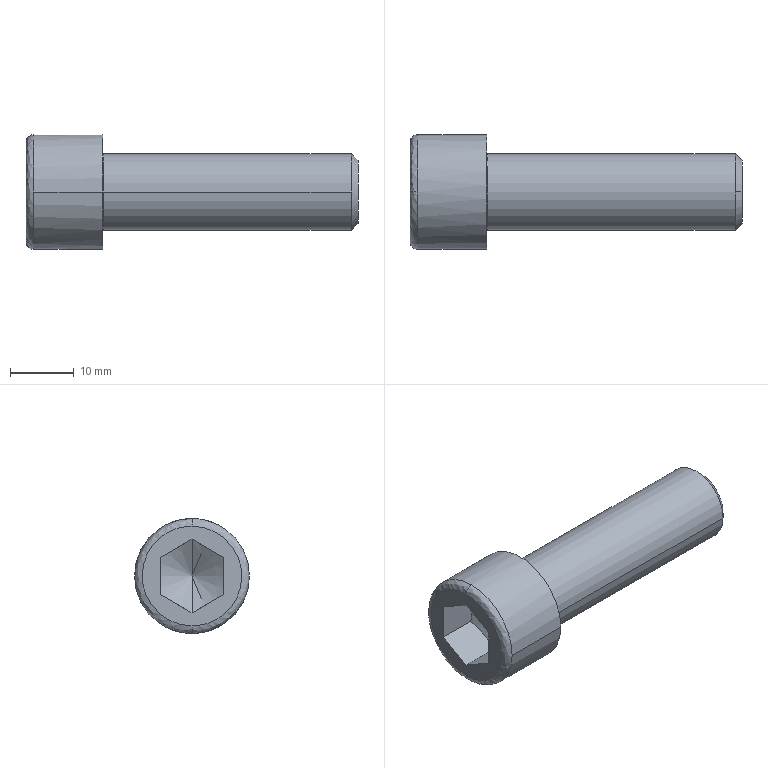Part | SolidWorks | features BaseBody 1 | 1 solid | 21 faces | box 52 x 18 x 18 mm | volume 6907 mm3 | plane 9 | spline 4 | cylinder 4 | cone 4 | commonest cylinder face diameters 12 x2 18 x2
STEP:
#1=CARTESIAN_POINT('',(0.,0.,6.1));
#2=VERTEX_POINT('',#1);
#3=CARTESIAN_POINT('',(0.,0.,-6.1));
#4=VERTEX_POINT('',#3);
#5=CARTESIAN_POINT('',(0.,0.,6.1));
#6=CARTESIAN_POINT('',(0.,0.1864,6.1));
#7=CARTESIAN_POINT('',(0.,0.4649,6.087));
#8=CARTESIAN_POINT('',(0.,0.788,6.05));
#9=CARTESIAN_POINT('',(0.,0.9492,6.026));
#10=CARTESIAN_POINT('',(0.,1.018,6.014));
#11=CARTESIAN_POINT('',(0.,1.064,6.007));
#12=CARTESIAN_POINT('',(0.,1.086,6.003));
#13=CARTESIAN_POINT('',(0.,1.304,5.962));
#14=CARTESIAN_POINT('',(0.,1.592,5.894));
#15=CARTESIAN_POINT('',(0.,1.921,5.791));
#16=CARTESIAN_POINT('',(0.,2.06,5.742));
#17=CARTESIAN_POINT('',(0.,2.153,5.708));
#18=CARTESIAN_POINT('',(0.,2.198,5.691));
#19=CARTESIAN_POINT('',(0.,2.437,5.596));
#20=CARTESIAN_POINT('',(0.,2.717,5.468));
#21=CARTESIAN_POINT('',(0.,2.987,5.32));
#22=CARTESIAN_POINT('',(0.,3.164,5.216));
#23=CARTESIAN_POINT('',(0.,3.25,5.163));
#24=CARTESIAN_POINT('',(0.,3.69,4.875));
#25=CARTESIAN_POINT('',(0.,4.016,4.611));
#26=CARTESIAN_POINT('',(0.,4.462,4.165));
#27=CARTESIAN_POINT('',(0.,4.673,3.931));
#28=CARTESIAN_POINT('',(0.,4.897,3.641));
#29=CARTESIAN_POINT('',(0.,4.988,3.512));
#30=CARTESIAN_POINT('',(0.,5.047,3.426));
#31=CARTESIAN_POINT('',(0.,5.077,3.381));
#32=CARTESIAN_POINT('',(0.,5.218,3.166));
#33=CARTESIAN_POINT('',(0.,5.374,2.9));
#34=CARTESIAN_POINT('',(0.,5.531,2.577));
#35=CARTESIAN_POINT('',(0.,5.593,2.436));
#36=CARTESIAN_POINT('',(0.,5.633,2.341));
#37=CARTESIAN_POINT('',(0.,5.654,2.291));
#38=CARTESIAN_POINT('',(0.,5.744,2.062));
#39=CARTESIAN_POINT('',(0.,5.84,1.782));
#40=CARTESIAN_POINT('',(0.,5.927,1.448));
#41=CARTESIAN_POINT('',(0.,5.965,1.28));
#42=CARTESIAN_POINT('',(0.,5.979,1.207));
#43=CARTESIAN_POINT('',(0.,5.989,1.159));
#44=CARTESIAN_POINT('',(0.,5.994,1.133));
#45=CARTESIAN_POINT('',(0.,6.066,0.7429));
#46=CARTESIAN_POINT('',(0.,6.1,0.3729));
#47=CARTESIAN_POINT('',(0.,6.1,-0.1865));
#48=CARTESIAN_POINT('',(0.,6.091,-0.3725));
#49=CARTESIAN_POINT('',(0.,6.066,-0.65));
#50=CARTESIAN_POINT('',(0.,6.05,-0.7884));
#51=CARTESIAN_POINT('',(0.,6.026,-0.9494));
#52=CARTESIAN_POINT('',(0.,6.014,-1.018));
#53=CARTESIAN_POINT('',(0.,6.007,-1.064));
#54=CARTESIAN_POINT('',(0.,6.003,-1.086));
#55=CARTESIAN_POINT('',(0.,5.962,-1.304));
#56=CARTESIAN_POINT('',(0.,5.894,-1.592));
#57=CARTESIAN_POINT('',(0.,5.791,-1.921));
#58=CARTESIAN_POINT('',(0.,5.742,-2.06));
#59=CARTESIAN_POINT('',(0.,5.708,-2.153));
#60=CARTESIAN_POINT('',(0.,5.691,-2.198));
#61=CARTESIAN_POINT('',(0.,5.596,-2.437));
#62=CARTESIAN_POINT('',(0.,5.468,-2.717));
#63=CARTESIAN_POINT('',(0.,5.32,-2.987));
#64=CARTESIAN_POINT('',(0.,5.216,-3.164));
#65=CARTESIAN_POINT('',(0.,5.163,-3.25));
#66=CARTESIAN_POINT('',(0.,4.875,-3.69));
#67=CARTESIAN_POINT('',(0.,4.611,-4.016));
#68=CARTESIAN_POINT('',(0.,4.165,-4.462));
#69=CARTESIAN_POINT('',(0.,3.931,-4.673));
#70=CARTESIAN_POINT('',(0.,3.641,-4.897));
#71=CARTESIAN_POINT('',(0.,3.512,-4.988));
#72=CARTESIAN_POINT('',(0.,3.426,-5.047));
#73=CARTESIAN_POINT('',(0.,3.381,-5.077));
#74=CARTESIAN_POINT('',(0.,3.166,-5.218));
#75=CARTESIAN_POINT('',(0.,2.9,-5.374));
#76=CARTESIAN_POINT('',(0.,2.577,-5.531));
#77=CARTESIAN_POINT('',(0.,2.436,-5.593));
#78=CARTESIAN_POINT('',(0.,2.341,-5.633));
#79=CARTESIAN_POINT('',(0.,2.291,-5.654));
#80=CARTESIAN_POINT('',(0.,2.062,-5.744));
#81=CARTESIAN_POINT('',(0.,1.782,-5.84));
#82=CARTESIAN_POINT('',(0.,1.448,-5.927));
#83=CARTESIAN_POINT('',(0.,1.28,-5.965));
#84=CARTESIAN_POINT('',(0.,1.207,-5.979));
#85=CARTESIAN_POINT('',(0.,1.159,-5.989));
#86=CARTESIAN_POINT('',(0.,1.133,-5.994));
#87=CARTESIAN_POINT('',(0.,0.7435,-6.066));
#88=CARTESIAN_POINT('',(0.,0.3728,-6.1));
#89=CARTESIAN_POINT('',(0.,0.,-6.1));
#90=B_SPLINE_CURVE_WITH_KNOTS('',3,(#5,#6,#7,#8,#9,#10,#11,#12,#13,#14,#15,#16,#17,#18,#19,#20,#21,#22,#23,#24,#25,#26,#27,#28,#29,#30,#31,#32,#33,#34,#35,#36,#37,#38,#39,#40,#41,#42,#43,#44,#45,#46,#47,#48,#49,#50,#51,#52,#53,#54,#55,#56,#57,#58,#59,#60,#61,#62,#63,#64,#65,#66,#67,#68,#69,#70,#71,#72,#73,#74,#75,#76,#77,#78,#79,#80,#81,#82,#83,#84,#85,#86,#87,#88,#89),.UNSPECIFIED.,.F.,.F.,(4,1,1,1,2,2,1,1,2,2,1,2,2,2,1,1,2,2,1,1,2,2,1,1,1,2,2,2,2,1,1,2,2,1,1,2,2,1,2,2,2,1,1,2,2,1,1,2,2,1,1,1,2,2,4),(0.75,0.7656,0.7734,0.7773,0.7793,0.7812,0.7969,0.8047,0.8086,0.8125,0.8281,0.8359,0.8437,0.875,0.8906,0.8984,0.9023,0.9063,0.9219,0.9297,0.9336,0.9375,0.9531,0.9609,0.9648,0.9668,0.9688,1.,1.016,1.023,1.027,1.029,1.031,1.047,1.055,1.059,1.063,1.078,1.086,1.094,1.125,1.141,1.148,1.152,1.156,1.172,1.18,1.184,1.188,1.203,1.211,1.215,1.217,1.219,1.25),.UNSPECIFIED.);
#91=EDGE_CURVE('',#2,#4,#90,.T.);
#92=ORIENTED_EDGE('',*,*,#91,.F.);
#93=CARTESIAN_POINT('',(0.1,0.,6.));
#94=VERTEX_POINT('',#93);
#95=CARTESIAN_POINT('',(0.1,0.,6.1));
#96=DIRECTION('',(0.,-1.,0.));
#97=DIRECTION('',(0.,0.,1.));
#98=AXIS2_PLACEMENT_3D('',#95,#96,#97);
#99=CIRCLE('',#98,0.1);
#100=EDGE_CURVE('',#2,#94,#99,.T.);
#101=ORIENTED_EDGE('',*,*,#100,.T.);
#102=CARTESIAN_POINT('',(0.1,6.,0.));
#103=VERTEX_POINT('',#102);
#104=CARTESIAN_POINT('',(0.1,0.,0.));
#105=DIRECTION('',(1.,0.,0.));
#106=DIRECTION('',(0.,1.,0.));
#107=AXIS2_PLACEMENT_3D('',#104,#105,#106);
#108=CIRCLE('',#107,6.);
#109=EDGE_CURVE('',#103,#94,#108,.T.);
#110=ORIENTED_EDGE('',*,*,#109,.F.);
#111=CARTESIAN_POINT('',(0.1,0.,-6.));
#112=VERTEX_POINT('',#111);
#113=CARTESIAN_POINT('',(0.1,0.,0.));
#114=DIRECTION('',(1.,0.,0.));
#115=DIRECTION('',(0.,1.,0.));
#116=AXIS2_PLACEMENT_3D('',#113,#114,#115);
#117=CIRCLE('',#116,6.);
#118=EDGE_CURVE('',#112,#103,#117,.T.);
#119=ORIENTED_EDGE('',*,*,#118,.F.);
#120=CARTESIAN_POINT('',(0.1,0.,-6.1));
#121=DIRECTION('',(0.,1.,0.));
#122=DIRECTION('',(0.,0.,-1.));
#123=AXIS2_PLACEMENT_3D('',#120,#121,#122);
#124=CIRCLE('',#123,0.1);
#125=EDGE_CURVE('',#4,#112,#124,.T.);
#126=ORIENTED_EDGE('',*,*,#125,.F.);
#127=EDGE_LOOP('',(#92,#101,#110,#119,#126));
#128=FACE_OUTER_BOUND('',#127,.T.);
#129=CARTESIAN_POINT('',(0.,0.,-6.1));
#130=CARTESIAN_POINT('',(0.,12.2,-6.1));
#131=CARTESIAN_POINT('',(0.,12.2,6.1));
#132=CARTESIAN_POINT('',(0.,0.,6.1));
#133=CARTESIAN_POINT('',(0.,0.,-6.041));
#134=CARTESIAN_POINT('',(0.,12.083,-6.041));
#135=CARTESIAN_POINT('',(0.,12.083,6.041));
#136=CARTESIAN_POINT('',(0.,0.,6.041));
#137=CARTESIAN_POINT('',(0.04142,0.,-6.));
#138=CARTESIAN_POINT('',(0.04142,12.,-6.));
#139=CARTESIAN_POINT('',(0.04142,12.,6.));
#140=CARTESIAN_POINT('',(0.04142,0.,6.));
#141=CARTESIAN_POINT('',(0.1,0.,-6.));
#142=CARTESIAN_POINT('',(0.1,12.,-6.));
#143=CARTESIAN_POINT('',(0.1,12.,6.));
#144=CARTESIAN_POINT('',(0.1,0.,6.));
#145=(BOUNDED_SURFACE()B_SPLINE_SURFACE(3,3,((#129,#130,#131,#132),(#133,#134,#135,#136),(#137,#138,#139,#140),(#141,#142,#143,#144)),.UNSPECIFIED.,.F.,.F.,.F.)B_SPLINE_SURFACE_WITH_KNOTS((4,4),(4,4),(0.,1.),(0.,1.),.UNSPECIFIED.)GEOMETRIC_REPRESENTATION_ITEM()RATIONAL_B_SPLINE_SURFACE(((1.,0.3333,0.3333,1.),(0.8047,0.2682,0.2682,0.8047),(0.8047,0.2682,0.2682,0.8047),(1.,0.3333,0.3333,1.)))REPRESENTATION_ITEM('')SURFACE());
#146=ADVANCED_FACE('',(#128),#145,.F.);
#147=CARTESIAN_POINT('',(-10.8,0.,9.));
#148=VERTEX_POINT('',#147);
#149=CARTESIAN_POINT('',(-10.8,-9.,0.));
#150=VERTEX_POINT('',#149);
#151=CARTESIAN_POINT('',(-10.8,0.,0.));
#152=DIRECTION('',(1.,0.,0.));
#153=DIRECTION('',(0.,1.,0.));
#154=AXIS2_PLACEMENT_3D('',#151,#152,#153);
#155=CIRCLE('',#154,9.);
#156=EDGE_CURVE('',#148,#150,#155,.T.);
#157=ORIENTED_EDGE('',*,*,#156,.F.);
#158=CARTESIAN_POINT('',(-12.,0.,7.8));
#159=VERTEX_POINT('',#158);
#160=CARTESIAN_POINT('',(-10.8,0.,7.8));
#161=DIRECTION('',(0.,-1.,0.));
#162=DIRECTION('',(0.,0.,1.));
#163=AXIS2_PLACEMENT_3D('',#160,#161,#162);
#164=CIRCLE('',#163,1.2);
#165=EDGE_CURVE('',#148,#159,#164,.T.);
#166=ORIENTED_EDGE('',*,*,#165,.T.);
#167=CARTESIAN_POINT('',(-12.,0.,-7.8));
#168=VERTEX_POINT('',#167);
#169=CARTESIAN_POINT('',(-12.,0.,7.8));
#170=CARTESIAN_POINT('',(-12.,-15.6,7.8));
#171=CARTESIAN_POINT('',(-12.,-15.6,-7.8));
#172=CARTESIAN_POINT('',(-12.,0.,-7.8));
#173=(BOUNDED_CURVE()B_SPLINE_CURVE(3,(#169,#170,#171,#172),.UNSPECIFIED.,.F.,.F.)B_SPLINE_CURVE_WITH_KNOTS((4,4),(0.25,0.75),.UNSPECIFIED.)CURVE()GEOMETRIC_REPRESENTATION_ITEM()RATIONAL_B_SPLINE_CURVE((1.,0.3333,0.3333,1.))REPRESENTATION_ITEM(''));
#174=EDGE_CURVE('',#159,#168,#173,.T.);
#175=ORIENTED_EDGE('',*,*,#174,.T.);
#176=CARTESIAN_POINT('',(-10.8,0.,-9.));
#177=VERTEX_POINT('',#176);
#178=CARTESIAN_POINT('',(-10.8,0.,-7.8));
#179=DIRECTION('',(0.,1.,0.));
#180=DIRECTION('',(0.,0.,-1.));
#181=AXIS2_PLACEMENT_3D('',#178,#179,#180);
#182=CIRCLE('',#181,1.2);
#183=EDGE_CURVE('',#177,#168,#182,.T.);
#184=ORIENTED_EDGE('',*,*,#183,.F.);
#185=CARTESIAN_POINT('',(-10.8,0.,0.));
#186=DIRECTION('',(1.,0.,0.));
#187=DIRECTION('',(0.,1.,0.));
#188=AXIS2_PLACEMENT_3D('',#185,#186,#187);
#189=CIRCLE('',#188,9.);
#190=EDGE_CURVE('',#150,#177,#189,.T.);
#191=ORIENTED_EDGE('',*,*,#190,.F.);
#192=EDGE_LOOP('',(#157,#166,#175,#184,#191));
#193=FACE_OUTER_BOUND('',#192,.T.);
#194=CARTESIAN_POINT('',(-10.8,0.,9.));
#195=CARTESIAN_POINT('',(-10.8,-18.,9.));
#196=CARTESIAN_POINT('',(-10.8,-18.,-9.));
#197=CARTESIAN_POINT('',(-10.8,0.,-9.));
#198=CARTESIAN_POINT('',(-11.503,0.,9.));
#199=CARTESIAN_POINT('',(-11.503,-18.,9.));
#200=CARTESIAN_POINT('',(-11.503,-18.,-9.));
#201=CARTESIAN_POINT('',(-11.503,0.,-9.));
#202=CARTESIAN_POINT('',(-12.,0.,8.503));
#203=CARTESIAN_POINT('',(-12.,-17.006,8.503));
#204=CARTESIAN_POINT('',(-12.,-17.006,-8.503));
#205=CARTESIAN_POINT('',(-12.,0.,-8.503));
#206=CARTESIAN_POINT('',(-12.,0.,7.8));
#207=CARTESIAN_POINT('',(-12.,-15.6,7.8));
#208=CARTESIAN_POINT('',(-12.,-15.6,-7.8));
#209=CARTESIAN_POINT('',(-12.,0.,-7.8));
#210=(BOUNDED_SURFACE()B_SPLINE_SURFACE(3,3,((#194,#195,#196,#197),(#198,#199,#200,#201),(#202,#203,#204,#205),(#206,#207,#208,#209)),.UNSPECIFIED.,.F.,.F.,.F.)B_SPLINE_SURFACE_WITH_KNOTS((4,4),(4,4),(0.,1.),(0.,1.),.UNSPECIFIED.)GEOMETRIC_REPRESENTATION_ITEM()RATIONAL_B_SPLINE_SURFACE(((1.,0.3333,0.3333,1.),(0.8047,0.2682,0.2682,0.8047),(0.8047,0.2682,0.2682,0.8047),(1.,0.3333,0.3333,1.)))REPRESENTATION_ITEM('')SURFACE());
#211=ADVANCED_FACE('',(#193),#210,.T.);
#212=ORIENTED_EDGE('',*,*,#109,.T.);
#213=CARTESIAN_POINT('',(0.1,-6.,0.));
#214=VERTEX_POINT('',#213);
#215=CARTESIAN_POINT('',(0.1,0.,0.));
#216=DIRECTION('',(1.,0.,0.));
#217=DIRECTION('',(0.,1.,0.));
#218=AXIS2_PLACEMENT_3D('',#215,#216,#217);
#219=CIRCLE('',#218,6.);
#220=EDGE_CURVE('',#94,#214,#219,.T.);
#221=ORIENTED_EDGE('',*,*,#220,.T.);
#222=CARTESIAN_POINT('',(38.926,-6.,0.));
#223=VERTEX_POINT('',#222);
#224=CARTESIAN_POINT('',(25.,-6.,0.));
#225=DIRECTION('',(1.,0.,0.));
#226=VECTOR('',#225,1000.);
#227=LINE('',#224,#226);
#228=EDGE_CURVE('',#214,#223,#227,.T.);
#229=ORIENTED_EDGE('',*,*,#228,.T.);
#230=CARTESIAN_POINT('',(38.926,0.,6.));
#231=VERTEX_POINT('',#230);
#232=CARTESIAN_POINT('',(38.926,0.,0.));
#233=DIRECTION('',(-1.,0.,0.));
#234=DIRECTION('',(0.,1.,0.));
#235=AXIS2_PLACEMENT_3D('',#232,#233,#234);
#236=CIRCLE('',#235,6.);
#237=EDGE_CURVE('',#223,#231,#236,.T.);
#238=ORIENTED_EDGE('',*,*,#237,.T.);
#239=CARTESIAN_POINT('',(38.926,6.,0.));
#240=VERTEX_POINT('',#239);
#241=CARTESIAN_POINT('',(38.926,0.,0.));
#242=DIRECTION('',(-1.,0.,0.));
#243=DIRECTION('',(0.,1.,0.));
#244=AXIS2_PLACEMENT_3D('',#241,#242,#243);
#245=CIRCLE('',#244,6.);
#246=EDGE_CURVE('',#231,#240,#245,.T.);
#247=ORIENTED_EDGE('',*,*,#246,.T.);
#248=CARTESIAN_POINT('',(25.,6.,0.));
#249=DIRECTION('',(1.,0.,0.));
#250=VECTOR('',#249,1000.);
#251=LINE('',#248,#250);
#252=EDGE_CURVE('',#103,#240,#251,.T.);
#253=ORIENTED_EDGE('',*,*,#252,.F.);
#254=EDGE_LOOP('',(#212,#221,#229,#238,#247,#253));
#255=FACE_OUTER_BOUND('',#254,.T.);
#256=CARTESIAN_POINT('',(25.,0.,0.));
#257=DIRECTION('',(1.,0.,0.));
#258=DIRECTION('',(0.,1.,0.));
#259=AXIS2_PLACEMENT_3D('',#256,#257,#258);
#260=CYLINDRICAL_SURFACE('',#259,6.);
#261=ADVANCED_FACE('',(#255),#260,.T.);
#262=CARTESIAN_POINT('',(40.,0.,4.926));
#263=VERTEX_POINT('',#262);
#264=CARTESIAN_POINT('',(40.,0.,-4.926));
#265=VERTEX_POINT('',#264);
#266=CARTESIAN_POINT('',(40.,0.,0.));
#267=DIRECTION('',(-1.,0.,0.));
#268=DIRECTION('',(0.,0.,1.));
#269=AXIS2_PLACEMENT_3D('',#266,#267,#268);
#270=CIRCLE('',#269,4.926);
#271=EDGE_CURVE('',#263,#265,#270,.T.);
#272=ORIENTED_EDGE('',*,*,#271,.T.);
#273=CARTESIAN_POINT('',(38.926,0.,-6.));
#274=VERTEX_POINT('',#273);
#275=CARTESIAN_POINT('',(38.926,0.,-6.));
#276=DIRECTION('',(-0.7071,0.,-0.7071));
#277=VECTOR('',#276,1000.);
#278=LINE('',#275,#277);
#279=EDGE_CURVE('',#265,#274,#278,.T.);
#280=ORIENTED_EDGE('',*,*,#279,.T.);
#281=CARTESIAN_POINT('',(38.926,0.,0.));
#282=DIRECTION('',(-1.,0.,0.));
#283=DIRECTION('',(0.,1.,0.));
#284=AXIS2_PLACEMENT_3D('',#281,#282,#283);
#285=CIRCLE('',#284,6.);
#286=EDGE_CURVE('',#240,#274,#285,.T.);
#287=ORIENTED_EDGE('',*,*,#286,.F.);
#288=ORIENTED_EDGE('',*,*,#246,.F.);
#289=CARTESIAN_POINT('',(38.926,0.,6.));
#290=DIRECTION('',(-0.7071,0.,0.7071));
#291=VECTOR('',#290,1000.);
#292=LINE('',#289,#291);
#293=EDGE_CURVE('',#263,#231,#292,.T.);
#294=ORIENTED_EDGE('',*,*,#293,.F.);
#295=EDGE_LOOP('',(#272,#280,#287,#288,#294));
#296=FACE_OUTER_BOUND('',#295,.T.);
#297=CARTESIAN_POINT('',(38.926,0.,0.));
#298=DIRECTION('',(-1.,0.,0.));
#299=DIRECTION('',(0.,0.,1.));
#300=AXIS2_PLACEMENT_3D('',#297,#298,#299);
#301=CONICAL_SURFACE('',#300,6.,0.7854);
#302=ADVANCED_FACE('',(#296),#301,.T.);
#303=CARTESIAN_POINT('',(-10.8,9.,0.));
#304=VERTEX_POINT('',#303);
#305=CARTESIAN_POINT('',(-10.8,0.,0.));
#306=DIRECTION('',(1.,0.,0.));
#307=DIRECTION('',(0.,1.,0.));
#308=AXIS2_PLACEMENT_3D('',#305,#306,#307);
#309=CIRCLE('',#308,9.);
#310=EDGE_CURVE('',#304,#148,#309,.T.);
#311=ORIENTED_EDGE('',*,*,#310,.T.);
#312=ORIENTED_EDGE('',*,*,#156,.T.);
#313=CARTESIAN_POINT('',(0.,-9.,0.));
#314=VERTEX_POINT('',#313);
#315=CARTESIAN_POINT('',(-6.,-9.,0.));
#316=DIRECTION('',(1.,0.,0.));
#317=VECTOR('',#316,1000.);
#318=LINE('',#315,#317);
#319=EDGE_CURVE('',#150,#314,#318,.T.);
#320=ORIENTED_EDGE('',*,*,#319,.T.);
#321=CARTESIAN_POINT('',(0.,9.,0.));
#322=VERTEX_POINT('',#321);
#323=CARTESIAN_POINT('',(0.,0.,0.));
#324=DIRECTION('',(1.,0.,0.));
#325=DIRECTION('',(0.,1.,0.));
#326=AXIS2_PLACEMENT_3D('',#323,#324,#325);
#327=CIRCLE('',#326,9.);
#328=EDGE_CURVE('',#322,#314,#327,.T.);
#329=ORIENTED_EDGE('',*,*,#328,.F.);
#330=CARTESIAN_POINT('',(-6.,9.,0.));
#331=DIRECTION('',(1.,0.,0.));
#332=VECTOR('',#331,1000.);
#333=LINE('',#330,#332);
#334=EDGE_CURVE('',#304,#322,#333,.T.);
#335=ORIENTED_EDGE('',*,*,#334,.F.);
#336=EDGE_LOOP('',(#311,#312,#320,#329,#335));
#337=FACE_OUTER_BOUND('',#336,.T.);
#338=CARTESIAN_POINT('',(-6.,0.,0.));
#339=DIRECTION('',(1.,0.,0.));
#340=DIRECTION('',(0.,1.,0.));
#341=AXIS2_PLACEMENT_3D('',#338,#339,#340);
#342=CYLINDRICAL_SURFACE('',#341,9.);
#343=ADVANCED_FACE('',(#337),#342,.T.);
#344=CARTESIAN_POINT('',(-2.667,0.,0.));
#345=VERTEX_POINT('',#344);
#346=CARTESIAN_POINT('',(-6.,0.,5.774));
#347=VERTEX_POINT('',#346);
#348=CARTESIAN_POINT('',(-6.02,0.,5.808));
#349=DIRECTION('',(-0.5,0.,0.866));
#350=VECTOR('',#349,1000.);
#351=LINE('',#348,#350);
#352=EDGE_CURVE('',#345,#347,#351,.T.);
#353=ORIENTED_EDGE('',*,*,#352,.F.);
#354=CARTESIAN_POINT('',(-6.,0.,-5.774));
#355=VERTEX_POINT('',#354);
#356=CARTESIAN_POINT('',(-6.02,0.,-5.808));
#357=DIRECTION('',(-0.5,0.,-0.866));
#358=VECTOR('',#357,1000.);
#359=LINE('',#356,#358);
#360=EDGE_CURVE('',#345,#355,#359,.T.);
#361=ORIENTED_EDGE('',*,*,#360,.T.);
#362=CARTESIAN_POINT('',(-6.,-5.,-2.887));
#363=VERTEX_POINT('',#362);
#364=CARTESIAN_POINT('',(-6.,0.,-5.774));
#365=CARTESIAN_POINT('',(-5.728,-0.8164,-5.302));
#366=CARTESIAN_POINT('',(-5.554,-1.645,-4.824));
#367=CARTESIAN_POINT('',(-5.553,-2.708,-4.21));
#368=CARTESIAN_POINT('',(-5.564,-2.921,-4.087));
#369=CARTESIAN_POINT('',(-5.604,-3.344,-3.843));
#370=CARTESIAN_POINT('',(-5.635,-3.554,-3.722));
#371=CARTESIAN_POINT('',(-5.751,-4.179,-3.361));
#372=CARTESIAN_POINT('',(-5.864,-4.591,-3.123));
#373=CARTESIAN_POINT('',(-6.,-5.,-2.887));
#374=B_SPLINE_CURVE_WITH_KNOTS('',3,(#364,#365,#366,#367,#368,#369,#370,#371,#372,#373),.UNSPECIFIED.,.F.,.F.,(4,2,2,2,4),(0.,0.002915,0.003644,0.004373,0.005831),.UNSPECIFIED.);
#375=EDGE_CURVE('',#355,#363,#374,.T.);
#376=ORIENTED_EDGE('',*,*,#375,.T.);
#377=CARTESIAN_POINT('',(-6.,-5.,2.887));
#378=VERTEX_POINT('',#377);
#379=CARTESIAN_POINT('',(-6.,-5.,-2.887));
#380=CARTESIAN_POINT('',(-5.728,-5.,-1.944));
#381=CARTESIAN_POINT('',(-5.554,-5.,-0.9872));
#382=CARTESIAN_POINT('',(-5.553,-5.,0.2399));
#383=CARTESIAN_POINT('',(-5.564,-5.,0.4865));
#384=CARTESIAN_POINT('',(-5.604,-5.,0.9743));
#385=CARTESIAN_POINT('',(-5.635,-5.,1.216));
#386=CARTESIAN_POINT('',(-5.751,-5.,1.939));
#387=CARTESIAN_POINT('',(-5.864,-5.,2.415));
#388=CARTESIAN_POINT('',(-6.,-5.,2.887));
#389=B_SPLINE_CURVE_WITH_KNOTS('',3,(#379,#380,#381,#382,#383,#384,#385,#386,#387,#388),.UNSPECIFIED.,.F.,.F.,(4,2,2,2,4),(0.,0.002915,0.003644,0.004373,0.005831),.UNSPECIFIED.);
#390=EDGE_CURVE('',#363,#378,#389,.T.);
#391=ORIENTED_EDGE('',*,*,#390,.T.);
#392=CARTESIAN_POINT('',(-6.,-5.,2.887));
#393=CARTESIAN_POINT('',(-5.728,-4.184,3.358));
#394=CARTESIAN_POINT('',(-5.554,-3.355,3.837));
#395=CARTESIAN_POINT('',(-5.553,-2.292,4.45));
#396=CARTESIAN_POINT('',(-5.564,-2.079,4.573));
#397=CARTESIAN_POINT('',(-5.604,-1.656,4.817));
#398=CARTESIAN_POINT('',(-5.635,-1.446,4.938));
#399=CARTESIAN_POINT('',(-5.751,-0.8208,5.3));
#400=CARTESIAN_POINT('',(-5.864,-0.4087,5.538));
#401=CARTESIAN_POINT('',(-6.,0.,5.774));
#402=B_SPLINE_CURVE_WITH_KNOTS('',3,(#392,#393,#394,#395,#396,#397,#398,#399,#400,#401),.UNSPECIFIED.,.F.,.F.,(4,2,2,2,4),(0.,0.002915,0.003644,0.004373,0.005831),.UNSPECIFIED.);
#403=EDGE_CURVE('',#378,#347,#402,.T.);
#404=ORIENTED_EDGE('',*,*,#403,.T.);
#405=EDGE_LOOP('',(#353,#361,#376,#391,#404));
#406=FACE_OUTER_BOUND('',#405,.T.);
#407=CARTESIAN_POINT('',(-6.02,0.,0.));
#408=DIRECTION('',(-1.,0.,0.));
#409=DIRECTION('',(0.,0.,1.));
#410=AXIS2_PLACEMENT_3D('',#407,#408,#409);
#411=CONICAL_SURFACE('',#410,5.808,1.047);
#412=ADVANCED_FACE('',(#406),#411,.F.);
#413=ORIENTED_EDGE('',*,*,#228,.F.);
#414=CARTESIAN_POINT('',(0.1,0.,0.));
#415=DIRECTION('',(1.,0.,0.));
#416=DIRECTION('',(0.,1.,0.));
#417=AXIS2_PLACEMENT_3D('',#414,#415,#416);
#418=CIRCLE('',#417,6.);
#419=EDGE_CURVE('',#214,#112,#418,.T.);
#420=ORIENTED_EDGE('',*,*,#419,.T.);
#421=ORIENTED_EDGE('',*,*,#118,.T.);
#422=ORIENTED_EDGE('',*,*,#252,.T.);
#423=ORIENTED_EDGE('',*,*,#286,.T.);
#424=CARTESIAN_POINT('',(38.926,0.,0.));
#425=DIRECTION('',(-1.,0.,0.));
#426=DIRECTION('',(0.,1.,0.));
#427=AXIS2_PLACEMENT_3D('',#424,#425,#426);
#428=CIRCLE('',#427,6.);
#429=EDGE_CURVE('',#274,#223,#428,.T.);
#430=ORIENTED_EDGE('',*,*,#429,.T.);
#431=EDGE_LOOP('',(#413,#420,#421,#422,#423,#430));
#432=FACE_OUTER_BOUND('',#431,.T.);
#433=CARTESIAN_POINT('',(25.,0.,0.));
#434=DIRECTION('',(1.,0.,0.));
#435=DIRECTION('',(0.,1.,0.));
#436=AXIS2_PLACEMENT_3D('',#433,#434,#435);
#437=CYLINDRICAL_SURFACE('',#436,6.);
#438=ADVANCED_FACE('',(#432),#437,.T.);
#439=ORIENTED_EDGE('',*,*,#100,.F.);
#440=CARTESIAN_POINT('',(0.,0.,-6.1));
#441=CARTESIAN_POINT('',(0.,-0.1864,-6.1));
#442=CARTESIAN_POINT('',(0.,-0.4649,-6.087));
#443=CARTESIAN_POINT('',(0.,-0.788,-6.05));
#444=CARTESIAN_POINT('',(0.,-0.9492,-6.026));
#445=CARTESIAN_POINT('',(0.,-1.018,-6.014));
#446=CARTESIAN_POINT('',(0.,-1.064,-6.007));
#447=CARTESIAN_POINT('',(0.,-1.086,-6.003));
#448=CARTESIAN_POINT('',(0.,-1.304,-5.962));
#449=CARTESIAN_POINT('',(0.,-1.592,-5.894));
#450=CARTESIAN_POINT('',(0.,-1.921,-5.791));
#451=CARTESIAN_POINT('',(0.,-2.06,-5.742));
#452=CARTESIAN_POINT('',(0.,-2.153,-5.708));
#453=CARTESIAN_POINT('',(0.,-2.198,-5.691));
#454=CARTESIAN_POINT('',(0.,-2.437,-5.596));
#455=CARTESIAN_POINT('',(0.,-2.717,-5.468));
#456=CARTESIAN_POINT('',(0.,-2.987,-5.32));
#457=CARTESIAN_POINT('',(0.,-3.164,-5.216));
#458=CARTESIAN_POINT('',(0.,-3.25,-5.163));
#459=CARTESIAN_POINT('',(0.,-3.69,-4.875));
#460=CARTESIAN_POINT('',(0.,-4.016,-4.611));
#461=CARTESIAN_POINT('',(0.,-4.462,-4.165));
#462=CARTESIAN_POINT('',(0.,-4.673,-3.931));
#463=CARTESIAN_POINT('',(0.,-4.897,-3.641));
#464=CARTESIAN_POINT('',(0.,-4.988,-3.512));
#465=CARTESIAN_POINT('',(0.,-5.047,-3.426));
#466=CARTESIAN_POINT('',(0.,-5.077,-3.381));
#467=CARTESIAN_POINT('',(0.,-5.218,-3.166));
#468=CARTESIAN_POINT('',(0.,-5.374,-2.9));
#469=CARTESIAN_POINT('',(0.,-5.531,-2.577));
#470=CARTESIAN_POINT('',(0.,-5.593,-2.436));
#471=CARTESIAN_POINT('',(0.,-5.633,-2.341));
#472=CARTESIAN_POINT('',(0.,-5.654,-2.291));
#473=CARTESIAN_POINT('',(0.,-5.744,-2.062));
#474=CARTESIAN_POINT('',(0.,-5.84,-1.782));
#475=CARTESIAN_POINT('',(0.,-5.927,-1.448));
#476=CARTESIAN_POINT('',(0.,-5.965,-1.28));
#477=CARTESIAN_POINT('',(0.,-5.979,-1.207));
#478=CARTESIAN_POINT('',(0.,-5.989,-1.159));
#479=CARTESIAN_POINT('',(0.,-5.994,-1.133));
#480=CARTESIAN_POINT('',(0.,-6.066,-0.7435));
#481=CARTESIAN_POINT('',(0.,-6.1,-0.3728));
#482=CARTESIAN_POINT('',(0.,-6.1,0.1864));
#483=CARTESIAN_POINT('',(0.,-6.087,0.4649));
#484=CARTESIAN_POINT('',(0.,-6.05,0.788));
#485=CARTESIAN_POINT('',(0.,-6.026,0.9492));
#486=CARTESIAN_POINT('',(0.,-6.014,1.018));
#487=CARTESIAN_POINT('',(0.,-6.007,1.064));
#488=CARTESIAN_POINT('',(0.,-6.003,1.086));
#489=CARTESIAN_POINT('',(0.,-5.962,1.304));
#490=CARTESIAN_POINT('',(0.,-5.894,1.592));
#491=CARTESIAN_POINT('',(0.,-5.791,1.921));
#492=CARTESIAN_POINT('',(0.,-5.742,2.06));
#493=CARTESIAN_POINT('',(0.,-5.708,2.153));
#494=CARTESIAN_POINT('',(0.,-5.691,2.198));
#495=CARTESIAN_POINT('',(0.,-5.596,2.437));
#496=CARTESIAN_POINT('',(0.,-5.468,2.717));
#497=CARTESIAN_POINT('',(0.,-5.32,2.987));
#498=CARTESIAN_POINT('',(0.,-5.216,3.164));
#499=CARTESIAN_POINT('',(0.,-5.163,3.25));
#500=CARTESIAN_POINT('',(0.,-4.875,3.69));
#501=CARTESIAN_POINT('',(0.,-4.611,4.016));
#502=CARTESIAN_POINT('',(0.,-4.165,4.462));
#503=CARTESIAN_POINT('',(0.,-3.931,4.673));
#504=CARTESIAN_POINT('',(0.,-3.641,4.897));
#505=CARTESIAN_POINT('',(0.,-3.512,4.988));
#506=CARTESIAN_POINT('',(0.,-3.426,5.047));
#507=CARTESIAN_POINT('',(0.,-3.381,5.077));
#508=CARTESIAN_POINT('',(0.,-3.166,5.218));
#509=CARTESIAN_POINT('',(0.,-2.9,5.374));
#510=CARTESIAN_POINT('',(0.,-2.577,5.531));
#511=CARTESIAN_POINT('',(0.,-2.436,5.593));
#512=CARTESIAN_POINT('',(0.,-2.341,5.633));
#513=CARTESIAN_POINT('',(0.,-2.291,5.654));
#514=CARTESIAN_POINT('',(0.,-2.062,5.744));
#515=CARTESIAN_POINT('',(0.,-1.782,5.84));
#516=CARTESIAN_POINT('',(0.,-1.448,5.927));
#517=CARTESIAN_POINT('',(0.,-1.28,5.965));
#518=CARTESIAN_POINT('',(0.,-1.207,5.979));
#519=CARTESIAN_POINT('',(0.,-1.159,5.989));
#520=CARTESIAN_POINT('',(0.,-1.133,5.994));
#521=CARTESIAN_POINT('',(0.,-0.7435,6.066));
#522=CARTESIAN_POINT('',(0.,-0.3728,6.1));
#523=CARTESIAN_POINT('',(0.,0.,6.1));
#524=B_SPLINE_CURVE_WITH_KNOTS('',3,(#440,#441,#442,#443,#444,#445,#446,#447,#448,#449,#450,#451,#452,#453,#454,#455,#456,#457,#458,#459,#460,#461,#462,#463,#464,#465,#466,#467,#468,#469,#470,#471,#472,#473,#474,#475,#476,#477,#478,#479,#480,#481,#482,#483,#484,#485,#486,#487,#488,#489,#490,#491,#492,#493,#494,#495,#496,#497,#498,#499,#500,#501,#502,#503,#504,#505,#506,#507,#508,#509,#510,#511,#512,#513,#514,#515,#516,#517,#518,#519,#520,#521,#522,#523),.UNSPECIFIED.,.F.,.F.,(4,1,1,1,2,2,1,1,2,2,1,2,2,2,1,1,2,2,1,1,2,2,1,1,1,2,2,2,1,1,1,2,2,1,1,2,2,1,2,2,2,1,1,2,2,1,1,2,2,1,1,1,2,2,4),(0.25,0.2656,0.2734,0.2773,0.2793,0.2813,0.2969,0.3047,0.3086,0.3125,0.3281,0.3359,0.3437,0.375,0.3906,0.3984,0.4023,0.4062,0.4219,0.4297,0.4336,0.4375,0.4531,0.4609,0.4648,0.4668,0.4687,0.5,0.5156,0.5234,0.5273,0.5293,0.5312,0.5469,0.5547,0.5586,0.5625,0.5781,0.5859,0.5937,0.625,0.6406,0.6484,0.6523,0.6562,0.6719,0.6797,0.6836,0.6875,0.7031,0.7109,0.7148,0.7168,0.7187,0.75),.UNSPECIFIED.);
#525=EDGE_CURVE('',#4,#2,#524,.T.);
#526=ORIENTED_EDGE('',*,*,#525,.F.);
#527=ORIENTED_EDGE('',*,*,#125,.T.);
#528=ORIENTED_EDGE('',*,*,#419,.F.);
#529=ORIENTED_EDGE('',*,*,#220,.F.);
#530=EDGE_LOOP('',(#439,#526,#527,#528,#529));
#531=FACE_OUTER_BOUND('',#530,.T.);
#532=CARTESIAN_POINT('',(0.,0.,6.1));
#533=CARTESIAN_POINT('',(0.,-12.2,6.1));
#534=CARTESIAN_POINT('',(0.,-12.2,-6.1));
#535=CARTESIAN_POINT('',(0.,0.,-6.1));
#536=CARTESIAN_POINT('',(0.,0.,6.041));
#537=CARTESIAN_POINT('',(0.,-12.083,6.041));
#538=CARTESIAN_POINT('',(0.,-12.083,-6.041));
#539=CARTESIAN_POINT('',(0.,0.,-6.041));
#540=CARTESIAN_POINT('',(0.04142,0.,6.));
#541=CARTESIAN_POINT('',(0.04142,-12.,6.));
#542=CARTESIAN_POINT('',(0.04142,-12.,-6.));
#543=CARTESIAN_POINT('',(0.04142,0.,-6.));
#544=CARTESIAN_POINT('',(0.1,0.,6.));
#545=CARTESIAN_POINT('',(0.1,-12.,6.));
#546=CARTESIAN_POINT('',(0.1,-12.,-6.));
#547=CARTESIAN_POINT('',(0.1,0.,-6.));
#548=(BOUNDED_SURFACE()B_SPLINE_SURFACE(3,3,((#532,#533,#534,#535),(#536,#537,#538,#539),(#540,#541,#542,#543),(#544,#545,#546,#547)),.UNSPECIFIED.,.F.,.F.,.T.)B_SPLINE_SURFACE_WITH_KNOTS((4,4),(4,4),(0.,1.),(0.,1.),.UNSPECIFIED.)GEOMETRIC_REPRESENTATION_ITEM()RATIONAL_B_SPLINE_SURFACE(((1.,0.3333,0.3333,1.),(0.8047,0.2682,0.2682,0.8047),(0.8047,0.2682,0.2682,0.8047),(1.,0.3333,0.3333,1.)))REPRESENTATION_ITEM('')SURFACE());
#549=ADVANCED_FACE('',(#531),#548,.F.);
#550=ORIENTED_EDGE('',*,*,#279,.F.);
#551=CARTESIAN_POINT('',(40.,0.,0.));
#552=DIRECTION('',(-1.,0.,0.));
#553=DIRECTION('',(0.,0.,1.));
#554=AXIS2_PLACEMENT_3D('',#551,#552,#553);
#555=CIRCLE('',#554,4.926);
#556=EDGE_CURVE('',#265,#263,#555,.T.);
#557=ORIENTED_EDGE('',*,*,#556,.T.);
#558=ORIENTED_EDGE('',*,*,#293,.T.);
#559=ORIENTED_EDGE('',*,*,#237,.F.);
#560=ORIENTED_EDGE('',*,*,#429,.F.);
#561=EDGE_LOOP('',(#550,#557,#558,#559,#560));
#562=FACE_OUTER_BOUND('',#561,.T.);
#563=CARTESIAN_POINT('',(38.926,0.,0.));
#564=DIRECTION('',(-1.,0.,0.));
#565=DIRECTION('',(0.,0.,1.));
#566=AXIS2_PLACEMENT_3D('',#563,#564,#565);
#567=CONICAL_SURFACE('',#566,6.,0.7854);
#568=ADVANCED_FACE('',(#562),#567,.T.);
#569=ORIENTED_EDGE('',*,*,#525,.T.);
#570=ORIENTED_EDGE('',*,*,#91,.T.);
#571=EDGE_LOOP('',(#569,#570));
#572=FACE_BOUND('',#571,.T.);
#573=ORIENTED_EDGE('',*,*,#328,.T.);
#574=CARTESIAN_POINT('',(0.,0.,0.));
#575=DIRECTION('',(1.,0.,0.));
#576=DIRECTION('',(0.,1.,0.));
#577=AXIS2_PLACEMENT_3D('',#574,#575,#576);
#578=CIRCLE('',#577,9.);
#579=EDGE_CURVE('',#314,#322,#578,.T.);
#580=ORIENTED_EDGE('',*,*,#579,.T.);
#581=EDGE_LOOP('',(#573,#580));
#582=FACE_OUTER_BOUND('',#581,.T.);
#583=CARTESIAN_POINT('',(0.,7.5,0.));
#584=DIRECTION('',(1.,0.,0.));
#585=DIRECTION('',(0.,1.,0.));
#586=AXIS2_PLACEMENT_3D('',#583,#584,#585);
#587=PLANE('',#586);
#588=ADVANCED_FACE('',(#572,#582),#587,.T.);
#589=ORIENTED_EDGE('',*,*,#271,.F.);
#590=ORIENTED_EDGE('',*,*,#556,.F.);
#591=EDGE_LOOP('',(#589,#590));
#592=FACE_OUTER_BOUND('',#591,.T.);
#593=CARTESIAN_POINT('',(40.,3.,0.));
#594=DIRECTION('',(1.,0.,0.));
#595=DIRECTION('',(0.,1.,0.));
#596=AXIS2_PLACEMENT_3D('',#593,#594,#595);
#597=PLANE('',#596);
#598=ADVANCED_FACE('',(#592),#597,.T.);
#599=ORIENTED_EDGE('',*,*,#319,.F.);
#600=ORIENTED_EDGE('',*,*,#190,.T.);
#601=CARTESIAN_POINT('',(-10.8,0.,0.));
#602=DIRECTION('',(1.,0.,0.));
#603=DIRECTION('',(0.,1.,0.));
#604=AXIS2_PLACEMENT_3D('',#601,#602,#603);
#605=CIRCLE('',#604,9.);
#606=EDGE_CURVE('',#177,#304,#605,.T.);
#607=ORIENTED_EDGE('',*,*,#606,.T.);
#608=ORIENTED_EDGE('',*,*,#334,.T.);
#609=ORIENTED_EDGE('',*,*,#579,.F.);
#610=EDGE_LOOP('',(#599,#600,#607,#608,#609));
#611=FACE_OUTER_BOUND('',#610,.T.);
#612=CARTESIAN_POINT('',(-6.,0.,0.));
#613=DIRECTION('',(1.,0.,0.));
#614=DIRECTION('',(0.,1.,0.));
#615=AXIS2_PLACEMENT_3D('',#612,#613,#614);
#616=CYLINDRICAL_SURFACE('',#615,9.);
#617=ADVANCED_FACE('',(#611),#616,.T.);
#618=ORIENTED_EDGE('',*,*,#165,.F.);
#619=ORIENTED_EDGE('',*,*,#310,.F.);
#620=ORIENTED_EDGE('',*,*,#606,.F.);
#621=ORIENTED_EDGE('',*,*,#183,.T.);
#622=CARTESIAN_POINT('',(-12.,0.,-7.8));
#623=CARTESIAN_POINT('',(-12.,15.6,-7.8));
#624=CARTESIAN_POINT('',(-12.,15.6,7.8));
#625=CARTESIAN_POINT('',(-12.,0.,7.8));
#626=(BOUNDED_CURVE()B_SPLINE_CURVE(3,(#622,#623,#624,#625),.UNSPECIFIED.,.F.,.F.)B_SPLINE_CURVE_WITH_KNOTS((4,4),(0.75,1.25),.UNSPECIFIED.)CURVE()GEOMETRIC_REPRESENTATION_ITEM()RATIONAL_B_SPLINE_CURVE((1.,0.3333,0.3333,1.))REPRESENTATION_ITEM(''));
#627=EDGE_CURVE('',#168,#159,#626,.T.);
#628=ORIENTED_EDGE('',*,*,#627,.T.);
#629=EDGE_LOOP('',(#618,#619,#620,#621,#628));
#630=FACE_OUTER_BOUND('',#629,.T.);
#631=CARTESIAN_POINT('',(-10.8,0.,-9.));
#632=CARTESIAN_POINT('',(-10.8,18.,-9.));
#633=CARTESIAN_POINT('',(-10.8,18.,9.));
#634=CARTESIAN_POINT('',(-10.8,0.,9.));
#635=CARTESIAN_POINT('',(-11.503,0.,-9.));
#636=CARTESIAN_POINT('',(-11.503,18.,-9.));
#637=CARTESIAN_POINT('',(-11.503,18.,9.));
#638=CARTESIAN_POINT('',(-11.503,0.,9.));
#639=CARTESIAN_POINT('',(-12.,0.,-8.503));
#640=CARTESIAN_POINT('',(-12.,17.006,-8.503));
#641=CARTESIAN_POINT('',(-12.,17.006,8.503));
#642=CARTESIAN_POINT('',(-12.,0.,8.503));
#643=CARTESIAN_POINT('',(-12.,0.,-7.8));
#644=CARTESIAN_POINT('',(-12.,15.6,-7.8));
#645=CARTESIAN_POINT('',(-12.,15.6,7.8));
#646=CARTESIAN_POINT('',(-12.,0.,7.8));
#647=(BOUNDED_SURFACE()B_SPLINE_SURFACE(3,3,((#631,#632,#633,#634),(#635,#636,#637,#638),(#639,#640,#641,#642),(#643,#644,#645,#646)),.UNSPECIFIED.,.F.,.F.,.T.)B_SPLINE_SURFACE_WITH_KNOTS((4,4),(4,4),(0.,1.),(0.,1.),.UNSPECIFIED.)GEOMETRIC_REPRESENTATION_ITEM()RATIONAL_B_SPLINE_SURFACE(((1.,0.3333,0.3333,1.),(0.8047,0.2682,0.2682,0.8047),(0.8047,0.2682,0.2682,0.8047),(1.,0.3333,0.3333,1.)))REPRESENTATION_ITEM('')SURFACE());
#648=ADVANCED_FACE('',(#630),#647,.T.);
#649=CARTESIAN_POINT('',(-12.,-5.,-2.887));
#650=VERTEX_POINT('',#649);
#651=CARTESIAN_POINT('',(-12.,0.,-5.774));
#652=VERTEX_POINT('',#651);
#653=CARTESIAN_POINT('',(-12.,-5.,-2.887));
#654=DIRECTION('',(0.,0.866,-0.5));
#655=VECTOR('',#654,1000.);
#656=LINE('',#653,#655);
#657=EDGE_CURVE('',#650,#652,#656,.T.);
#658=ORIENTED_EDGE('',*,*,#657,.T.);
#659=CARTESIAN_POINT('',(-12.,5.,-2.887));
#660=VERTEX_POINT('',#659);
#661=CARTESIAN_POINT('',(-12.,0.,-5.774));
#662=DIRECTION('',(0.,0.866,0.5));
#663=VECTOR('',#662,1000.);
#664=LINE('',#661,#663);
#665=EDGE_CURVE('',#652,#660,#664,.T.);
#666=ORIENTED_EDGE('',*,*,#665,.T.);
#667=CARTESIAN_POINT('',(-12.,5.,2.887));
#668=VERTEX_POINT('',#667);
#669=CARTESIAN_POINT('',(-12.,5.,0.));
#670=DIRECTION('',(0.,0.,1.));
#671=VECTOR('',#670,1000.);
#672=LINE('',#669,#671);
#673=EDGE_CURVE('',#660,#668,#672,.T.);
#674=ORIENTED_EDGE('',*,*,#673,.T.);
#675=CARTESIAN_POINT('',(-12.,0.,5.774));
#676=VERTEX_POINT('',#675);
#677=CARTESIAN_POINT('',(-12.,5.,2.887));
#678=DIRECTION('',(0.,-0.866,0.5));
#679=VECTOR('',#678,1000.);
#680=LINE('',#677,#679);
#681=EDGE_CURVE('',#668,#676,#680,.T.);
#682=ORIENTED_EDGE('',*,*,#681,.T.);
#683=CARTESIAN_POINT('',(-12.,-5.,2.887));
#684=VERTEX_POINT('',#683);
#685=CARTESIAN_POINT('',(-12.,0.,5.774));
#686=DIRECTION('',(0.,-0.866,-0.5));
#687=VECTOR('',#686,1000.);
#688=LINE('',#685,#687);
#689=EDGE_CURVE('',#676,#684,#688,.T.);
#690=ORIENTED_EDGE('',*,*,#689,.T.);
#691=CARTESIAN_POINT('',(-12.,-5.,0.));
#692=DIRECTION('',(0.,0.,-1.));
#693=VECTOR('',#692,1000.);
#694=LINE('',#691,#693);
#695=EDGE_CURVE('',#684,#650,#694,.T.);
#696=ORIENTED_EDGE('',*,*,#695,.T.);
#697=EDGE_LOOP('',(#658,#666,#674,#682,#690,#696));
#698=FACE_BOUND('',#697,.T.);
#699=ORIENTED_EDGE('',*,*,#627,.F.);
#700=ORIENTED_EDGE('',*,*,#174,.F.);
#701=EDGE_LOOP('',(#699,#700));
#702=FACE_OUTER_BOUND('',#701,.T.);
#703=CARTESIAN_POINT('',(-12.,7.387,0.));
#704=DIRECTION('',(-1.,0.,0.));
#705=DIRECTION('',(0.,-1.,0.));
#706=AXIS2_PLACEMENT_3D('',#703,#704,#705);
#707=PLANE('',#706);
#708=ADVANCED_FACE('',(#698,#702),#707,.T.);
#709=CARTESIAN_POINT('',(-6.,5.,-2.887));
#710=VERTEX_POINT('',#709);
#711=CARTESIAN_POINT('',(-12.,5.,-2.887));
#712=DIRECTION('',(1.,0.,0.));
#713=VECTOR('',#712,1000.);
#714=LINE('',#711,#713);
#715=EDGE_CURVE('',#660,#710,#714,.T.);
#716=ORIENTED_EDGE('',*,*,#715,.F.);
#717=ORIENTED_EDGE('',*,*,#665,.F.);
#718=CARTESIAN_POINT('',(-12.,0.,-5.774));
#719=DIRECTION('',(-1.,0.,0.));
#720=VECTOR('',#719,1000.);
#721=LINE('',#718,#720);
#722=EDGE_CURVE('',#355,#652,#721,.T.);
#723=ORIENTED_EDGE('',*,*,#722,.F.);
#724=CARTESIAN_POINT('',(-6.,5.,-2.887));
#725=CARTESIAN_POINT('',(-5.728,4.184,-3.358));
#726=CARTESIAN_POINT('',(-5.554,3.355,-3.837));
#727=CARTESIAN_POINT('',(-5.553,2.292,-4.45));
#728=CARTESIAN_POINT('',(-5.564,2.079,-4.573));
#729=CARTESIAN_POINT('',(-5.604,1.656,-4.817));
#730=CARTESIAN_POINT('',(-5.635,1.446,-4.938));
#731=CARTESIAN_POINT('',(-5.751,0.8208,-5.3));
#732=CARTESIAN_POINT('',(-5.864,0.4087,-5.538));
#733=CARTESIAN_POINT('',(-6.,0.,-5.774));
#734=B_SPLINE_CURVE_WITH_KNOTS('',3,(#724,#725,#726,#727,#728,#729,#730,#731,#732,#733),.UNSPECIFIED.,.F.,.F.,(4,2,2,2,4),(0.,0.002915,0.003644,0.004373,0.005831),.UNSPECIFIED.);
#735=EDGE_CURVE('',#710,#355,#734,.T.);
#736=ORIENTED_EDGE('',*,*,#735,.F.);
#737=EDGE_LOOP('',(#716,#717,#723,#736));
#738=FACE_OUTER_BOUND('',#737,.T.);
#739=CARTESIAN_POINT('',(-12.,5.,-2.887));
#740=DIRECTION('',(0.,0.5,-0.866));
#741=DIRECTION('',(0.,0.866,0.5));
#742=AXIS2_PLACEMENT_3D('',#739,#740,#741);
#743=PLANE('',#742);
#744=ADVANCED_FACE('',(#738),#743,.F.);
#745=ORIENTED_EDGE('',*,*,#722,.T.);
#746=ORIENTED_EDGE('',*,*,#657,.F.);
#747=CARTESIAN_POINT('',(-12.,-5.,-2.887));
#748=DIRECTION('',(-1.,0.,0.));
#749=VECTOR('',#748,1000.);
#750=LINE('',#747,#749);
#751=EDGE_CURVE('',#363,#650,#750,.T.);
#752=ORIENTED_EDGE('',*,*,#751,.F.);
#753=ORIENTED_EDGE('',*,*,#375,.F.);
#754=EDGE_LOOP('',(#745,#746,#752,#753));
#755=FACE_OUTER_BOUND('',#754,.T.);
#756=CARTESIAN_POINT('',(-12.,0.,-5.774));
#757=DIRECTION('',(0.,-0.5,-0.866));
#758=DIRECTION('',(0.,0.866,-0.5));
#759=AXIS2_PLACEMENT_3D('',#756,#757,#758);
#760=PLANE('',#759);
#761=ADVANCED_FACE('',(#755),#760,.F.);
#762=ORIENTED_EDGE('',*,*,#751,.T.);
#763=ORIENTED_EDGE('',*,*,#695,.F.);
#764=CARTESIAN_POINT('',(-12.,-5.,2.887));
#765=DIRECTION('',(-1.,0.,0.));
#766=VECTOR('',#765,1000.);
#767=LINE('',#764,#766);
#768=EDGE_CURVE('',#378,#684,#767,.T.);
#769=ORIENTED_EDGE('',*,*,#768,.F.);
#770=ORIENTED_EDGE('',*,*,#390,.F.);
#771=EDGE_LOOP('',(#762,#763,#769,#770));
#772=FACE_OUTER_BOUND('',#771,.T.);
#773=CARTESIAN_POINT('',(-12.,-5.,-2.887));
#774=DIRECTION('',(0.,-1.,0.));
#775=DIRECTION('',(0.,0.,-1.));
#776=AXIS2_PLACEMENT_3D('',#773,#774,#775);
#777=PLANE('',#776);
#778=ADVANCED_FACE('',(#772),#777,.F.);
#779=ORIENTED_EDGE('',*,*,#768,.T.);
#780=ORIENTED_EDGE('',*,*,#689,.F.);
#781=CARTESIAN_POINT('',(-12.,0.,5.774));
#782=DIRECTION('',(-1.,0.,0.));
#783=VECTOR('',#782,1000.);
#784=LINE('',#781,#783);
#785=EDGE_CURVE('',#347,#676,#784,.T.);
#786=ORIENTED_EDGE('',*,*,#785,.F.);
#787=ORIENTED_EDGE('',*,*,#403,.F.);
#788=EDGE_LOOP('',(#779,#780,#786,#787));
#789=FACE_OUTER_BOUND('',#788,.T.);
#790=CARTESIAN_POINT('',(-12.,-5.,2.887));
#791=DIRECTION('',(0.,-0.5,0.866));
#792=DIRECTION('',(0.,-0.866,-0.5));
#793=AXIS2_PLACEMENT_3D('',#790,#791,#792);
#794=PLANE('',#793);
#795=ADVANCED_FACE('',(#789),#794,.F.);
#796=ORIENTED_EDGE('',*,*,#785,.T.);
#797=ORIENTED_EDGE('',*,*,#681,.F.);
#798=CARTESIAN_POINT('',(-6.,5.,2.887));
#799=VERTEX_POINT('',#798);
#800=CARTESIAN_POINT('',(-12.,5.,2.887));
#801=DIRECTION('',(-1.,0.,0.));
#802=VECTOR('',#801,1000.);
#803=LINE('',#800,#802);
#804=EDGE_CURVE('',#799,#668,#803,.T.);
#805=ORIENTED_EDGE('',*,*,#804,.F.);
#806=CARTESIAN_POINT('',(-6.,0.,5.774));
#807=CARTESIAN_POINT('',(-5.728,0.8164,5.302));
#808=CARTESIAN_POINT('',(-5.554,1.645,4.824));
#809=CARTESIAN_POINT('',(-5.553,2.708,4.21));
#810=CARTESIAN_POINT('',(-5.564,2.921,4.087));
#811=CARTESIAN_POINT('',(-5.604,3.344,3.843));
#812=CARTESIAN_POINT('',(-5.635,3.554,3.722));
#813=CARTESIAN_POINT('',(-5.751,4.179,3.361));
#814=CARTESIAN_POINT('',(-5.864,4.591,3.123));
#815=CARTESIAN_POINT('',(-6.,5.,2.887));
#816=B_SPLINE_CURVE_WITH_KNOTS('',3,(#806,#807,#808,#809,#810,#811,#812,#813,#814,#815),.UNSPECIFIED.,.F.,.F.,(4,2,2,2,4),(0.,0.002915,0.003644,0.004373,0.005831),.UNSPECIFIED.);
#817=EDGE_CURVE('',#347,#799,#816,.T.);
#818=ORIENTED_EDGE('',*,*,#817,.F.);
#819=EDGE_LOOP('',(#796,#797,#805,#818));
#820=FACE_OUTER_BOUND('',#819,.T.);
#821=CARTESIAN_POINT('',(-12.,0.,5.774));
#822=DIRECTION('',(0.,0.5,0.866));
#823=DIRECTION('',(0.,-0.866,0.5));
#824=AXIS2_PLACEMENT_3D('',#821,#822,#823);
#825=PLANE('',#824);
#826=ADVANCED_FACE('',(#820),#825,.F.);
#827=ORIENTED_EDGE('',*,*,#804,.T.);
#828=ORIENTED_EDGE('',*,*,#673,.F.);
#829=ORIENTED_EDGE('',*,*,#715,.T.);
#830=CARTESIAN_POINT('',(-6.,5.,2.887));
#831=CARTESIAN_POINT('',(-5.728,5.,1.944));
#832=CARTESIAN_POINT('',(-5.554,5.,0.9872));
#833=CARTESIAN_POINT('',(-5.553,5.,-0.2399));
#834=CARTESIAN_POINT('',(-5.564,5.,-0.4865));
#835=CARTESIAN_POINT('',(-5.604,5.,-0.9743));
#836=CARTESIAN_POINT('',(-5.635,5.,-1.216));
#837=CARTESIAN_POINT('',(-5.751,5.,-1.939));
#838=CARTESIAN_POINT('',(-5.864,5.,-2.415));
#839=CARTESIAN_POINT('',(-6.,5.,-2.887));
#840=B_SPLINE_CURVE_WITH_KNOTS('',3,(#830,#831,#832,#833,#834,#835,#836,#837,#838,#839),.UNSPECIFIED.,.F.,.F.,(4,2,2,2,4),(0.,0.002915,0.003644,0.004373,0.005831),.UNSPECIFIED.);
#841=EDGE_CURVE('',#799,#710,#840,.T.);
#842=ORIENTED_EDGE('',*,*,#841,.F.);
#843=EDGE_LOOP('',(#827,#828,#829,#842));
#844=FACE_OUTER_BOUND('',#843,.T.);
#845=CARTESIAN_POINT('',(-12.,5.,2.887));
#846=DIRECTION('',(0.,1.,0.));
#847=DIRECTION('',(0.,0.,1.));
#848=AXIS2_PLACEMENT_3D('',#845,#846,#847);
#849=PLANE('',#848);
#850=ADVANCED_FACE('',(#844),#849,.F.);
#851=ORIENTED_EDGE('',*,*,#360,.F.);
#852=ORIENTED_EDGE('',*,*,#352,.T.);
#853=ORIENTED_EDGE('',*,*,#817,.T.);
#854=ORIENTED_EDGE('',*,*,#841,.T.);
#855=ORIENTED_EDGE('',*,*,#735,.T.);
#856=EDGE_LOOP('',(#851,#852,#853,#854,#855));
#857=FACE_OUTER_BOUND('',#856,.T.);
#858=CARTESIAN_POINT('',(-6.02,0.,0.));
#859=DIRECTION('',(-1.,0.,0.));
#860=DIRECTION('',(0.,0.,1.));
#861=AXIS2_PLACEMENT_3D('',#858,#859,#860);
#862=CONICAL_SURFACE('',#861,5.808,1.047);
#863=ADVANCED_FACE('',(#857),#862,.F.);
#864=CLOSED_SHELL('',(#146,#211,#261,#302,#343,#412,#438,#549,#568,#588,#598,#617,#648,#708,#744,#761,#778,#795,#826,#850,#863));
#865=MANIFOLD_SOLID_BREP('',#864);
#866=CARTESIAN_POINT('',(0.,0.,0.));
#867=DIRECTION('',(0.,0.,1.));
#868=DIRECTION('',(1.,0.,0.));
#869=AXIS2_PLACEMENT_3D('',#866,#867,#868);
#870=(LENGTH_UNIT()NAMED_UNIT(*)SI_UNIT(.MILLI.,.METRE.));
#871=UNCERTAINTY_MEASURE_WITH_UNIT(LENGTH_MEASURE(0.00001),#870,'','');
#872=(NAMED_UNIT(*)PLANE_ANGLE_UNIT()SI_UNIT($,.RADIAN.));
#873=(NAMED_UNIT(*)SI_UNIT($,.STERADIAN.)SOLID_ANGLE_UNIT());
#874=(GEOMETRIC_REPRESENTATION_CONTEXT(3)GLOBAL_UNCERTAINTY_ASSIGNED_CONTEXT((#871))GLOBAL_UNIT_ASSIGNED_CONTEXT((#870,#872,#873))REPRESENTATION_CONTEXT('',''));
#875=ADVANCED_BREP_SHAPE_REPRESENTATION('',(#865,#869),#874);